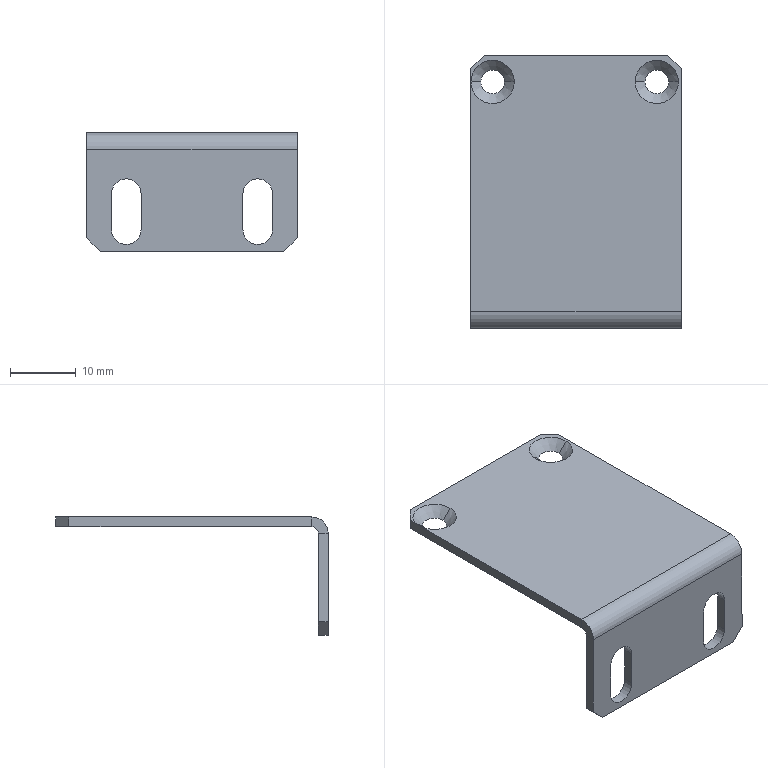Part | STEP file | FBDS-CS-034 | 1 solid | 32 faces | box 32 x 41.5 x 18 mm | volume 2551 mm3 | plane 20 | cylinder 8 | cone 4 | commonest cylinder face diameters 4.5 x6 2 x1 5 x1
STEP:
#1=CARTESIAN_POINT('',(-7.75,-21.5,-9.25));
#2=VERTEX_POINT('',#1);
#3=CARTESIAN_POINT('',(-10.,-21.5,-7.));
#4=VERTEX_POINT('',#3);
#5=CARTESIAN_POINT('',(-10.,-21.5,-9.25));
#6=DIRECTION('',(0.,-1.,0.));
#7=DIRECTION('',(0.,0.,-1.));
#8=AXIS2_PLACEMENT_3D('',#5,#6,#7);
#9=CIRCLE('',#8,2.25);
#10=EDGE_CURVE('',#2,#4,#9,.T.);
#11=ORIENTED_EDGE('',*,*,#10,.T.);
#12=CARTESIAN_POINT('',(-10.,-20.,-7.));
#13=VERTEX_POINT('',#12);
#14=CARTESIAN_POINT('',(-10.,-20.,-7.));
#15=DIRECTION('',(0.,1.,0.));
#16=VECTOR('',#15,1000.);
#17=LINE('',#14,#16);
#18=EDGE_CURVE('',#4,#13,#17,.T.);
#19=ORIENTED_EDGE('',*,*,#18,.T.);
#20=CARTESIAN_POINT('',(-7.75,-20.,-9.25));
#21=VERTEX_POINT('',#20);
#22=CARTESIAN_POINT('',(-10.,-20.,-9.25));
#23=DIRECTION('',(0.,1.,0.));
#24=DIRECTION('',(0.,0.,1.));
#25=AXIS2_PLACEMENT_3D('',#22,#23,#24);
#26=CIRCLE('',#25,2.25);
#27=EDGE_CURVE('',#13,#21,#26,.T.);
#28=ORIENTED_EDGE('',*,*,#27,.T.);
#29=CARTESIAN_POINT('',(-7.75,-30.1,-9.25));
#30=DIRECTION('',(0.,-1.,0.));
#31=VECTOR('',#30,1000.);
#32=LINE('',#29,#31);
#33=EDGE_CURVE('',#21,#2,#32,.T.);
#34=ORIENTED_EDGE('',*,*,#33,.T.);
#35=EDGE_LOOP('',(#11,#19,#28,#34));
#36=FACE_OUTER_BOUND('',#35,.T.);
#37=CARTESIAN_POINT('',(-10.,-20.,-9.25));
#38=DIRECTION('',(0.,1.,0.));
#39=DIRECTION('',(0.,0.,1.));
#40=AXIS2_PLACEMENT_3D('',#37,#38,#39);
#41=CYLINDRICAL_SURFACE('',#40,2.25);
#42=ADVANCED_FACE('',(#36),#41,.F.);
#43=CARTESIAN_POINT('',(12.25,-21.5,-9.25));
#44=VERTEX_POINT('',#43);
#45=CARTESIAN_POINT('',(10.,-21.5,-7.));
#46=VERTEX_POINT('',#45);
#47=CARTESIAN_POINT('',(10.,-21.5,-9.25));
#48=DIRECTION('',(0.,-1.,0.));
#49=DIRECTION('',(0.,0.,-1.));
#50=AXIS2_PLACEMENT_3D('',#47,#48,#49);
#51=CIRCLE('',#50,2.25);
#52=EDGE_CURVE('',#44,#46,#51,.T.);
#53=ORIENTED_EDGE('',*,*,#52,.T.);
#54=CARTESIAN_POINT('',(10.,-20.,-7.));
#55=VERTEX_POINT('',#54);
#56=CARTESIAN_POINT('',(10.,-20.,-7.));
#57=DIRECTION('',(0.,1.,0.));
#58=VECTOR('',#57,1000.);
#59=LINE('',#56,#58);
#60=EDGE_CURVE('',#46,#55,#59,.T.);
#61=ORIENTED_EDGE('',*,*,#60,.T.);
#62=CARTESIAN_POINT('',(12.25,-20.,-9.25));
#63=VERTEX_POINT('',#62);
#64=CARTESIAN_POINT('',(10.,-20.,-9.25));
#65=DIRECTION('',(0.,1.,0.));
#66=DIRECTION('',(0.,0.,1.));
#67=AXIS2_PLACEMENT_3D('',#64,#65,#66);
#68=CIRCLE('',#67,2.25);
#69=EDGE_CURVE('',#55,#63,#68,.T.);
#70=ORIENTED_EDGE('',*,*,#69,.T.);
#71=CARTESIAN_POINT('',(12.25,-30.1,-9.25));
#72=DIRECTION('',(0.,-1.,0.));
#73=VECTOR('',#72,1000.);
#74=LINE('',#71,#73);
#75=EDGE_CURVE('',#63,#44,#74,.T.);
#76=ORIENTED_EDGE('',*,*,#75,.T.);
#77=EDGE_LOOP('',(#53,#61,#70,#76));
#78=FACE_OUTER_BOUND('',#77,.T.);
#79=CARTESIAN_POINT('',(10.,-20.,-9.25));
#80=DIRECTION('',(0.,1.,0.));
#81=DIRECTION('',(0.,0.,1.));
#82=AXIS2_PLACEMENT_3D('',#79,#80,#81);
#83=CYLINDRICAL_SURFACE('',#82,2.25);
#84=ADVANCED_FACE('',(#78),#83,.F.);
#85=CARTESIAN_POINT('',(-10.9,16.,-1.5));
#86=VERTEX_POINT('',#85);
#87=CARTESIAN_POINT('',(-14.5,16.,-1.5));
#88=VERTEX_POINT('',#87);
#89=CARTESIAN_POINT('',(-12.7,16.,-1.5));
#90=DIRECTION('',(0.,0.,-1.));
#91=DIRECTION('',(-1.,0.,0.));
#92=AXIS2_PLACEMENT_3D('',#89,#90,#91);
#93=CIRCLE('',#92,1.8);
#94=EDGE_CURVE('',#86,#88,#93,.T.);
#95=ORIENTED_EDGE('',*,*,#94,.T.);
#96=CARTESIAN_POINT('',(-16.,16.,0.));
#97=VERTEX_POINT('',#96);
#98=CARTESIAN_POINT('',(-16.,16.,0.));
#99=DIRECTION('',(-0.7071,0.,0.7071));
#100=VECTOR('',#99,1000.);
#101=LINE('',#98,#100);
#102=EDGE_CURVE('',#88,#97,#101,.T.);
#103=ORIENTED_EDGE('',*,*,#102,.T.);
#104=CARTESIAN_POINT('',(-9.4,16.,0.));
#105=VERTEX_POINT('',#104);
#106=CARTESIAN_POINT('',(-12.7,16.,0.));
#107=DIRECTION('',(0.,0.,1.));
#108=DIRECTION('',(1.,0.,0.));
#109=AXIS2_PLACEMENT_3D('',#106,#107,#108);
#110=CIRCLE('',#109,3.3);
#111=EDGE_CURVE('',#97,#105,#110,.T.);
#112=ORIENTED_EDGE('',*,*,#111,.T.);
#113=CARTESIAN_POINT('',(-9.4,16.,0.));
#114=DIRECTION('',(0.7071,0.,0.7071));
#115=VECTOR('',#114,1000.);
#116=LINE('',#113,#115);
#117=EDGE_CURVE('',#86,#105,#116,.T.);
#118=ORIENTED_EDGE('',*,*,#117,.F.);
#119=EDGE_LOOP('',(#95,#103,#112,#118));
#120=FACE_OUTER_BOUND('',#119,.T.);
#121=CARTESIAN_POINT('',(-12.7,16.,0.));
#122=DIRECTION('',(0.,0.,1.));
#123=DIRECTION('',(1.,0.,0.));
#124=AXIS2_PLACEMENT_3D('',#121,#122,#123);
#125=CONICAL_SURFACE('',#124,3.3,0.7854);
#126=ADVANCED_FACE('',(#120),#125,.F.);
#127=CARTESIAN_POINT('',(14.1,16.,-1.5));
#128=VERTEX_POINT('',#127);
#129=CARTESIAN_POINT('',(10.5,16.,-1.5));
#130=VERTEX_POINT('',#129);
#131=CARTESIAN_POINT('',(12.3,16.,-1.5));
#132=DIRECTION('',(0.,0.,-1.));
#133=DIRECTION('',(-1.,0.,0.));
#134=AXIS2_PLACEMENT_3D('',#131,#132,#133);
#135=CIRCLE('',#134,1.8);
#136=EDGE_CURVE('',#128,#130,#135,.T.);
#137=ORIENTED_EDGE('',*,*,#136,.T.);
#138=CARTESIAN_POINT('',(9.,16.,0.));
#139=VERTEX_POINT('',#138);
#140=CARTESIAN_POINT('',(9.,16.,0.));
#141=DIRECTION('',(-0.7071,0.,0.7071));
#142=VECTOR('',#141,1000.);
#143=LINE('',#140,#142);
#144=EDGE_CURVE('',#130,#139,#143,.T.);
#145=ORIENTED_EDGE('',*,*,#144,.T.);
#146=CARTESIAN_POINT('',(15.6,16.,0.));
#147=VERTEX_POINT('',#146);
#148=CARTESIAN_POINT('',(12.3,16.,0.));
#149=DIRECTION('',(0.,0.,1.));
#150=DIRECTION('',(1.,0.,0.));
#151=AXIS2_PLACEMENT_3D('',#148,#149,#150);
#152=CIRCLE('',#151,3.3);
#153=EDGE_CURVE('',#139,#147,#152,.T.);
#154=ORIENTED_EDGE('',*,*,#153,.T.);
#155=CARTESIAN_POINT('',(15.6,16.,0.));
#156=DIRECTION('',(0.7071,0.,0.7071));
#157=VECTOR('',#156,1000.);
#158=LINE('',#155,#157);
#159=EDGE_CURVE('',#128,#147,#158,.T.);
#160=ORIENTED_EDGE('',*,*,#159,.F.);
#161=EDGE_LOOP('',(#137,#145,#154,#160));
#162=FACE_OUTER_BOUND('',#161,.T.);
#163=CARTESIAN_POINT('',(12.3,16.,0.));
#164=DIRECTION('',(0.,0.,1.));
#165=DIRECTION('',(1.,0.,0.));
#166=AXIS2_PLACEMENT_3D('',#163,#164,#165);
#167=CONICAL_SURFACE('',#166,3.3,0.7854);
#168=ADVANCED_FACE('',(#162),#167,.F.);
#169=CARTESIAN_POINT('',(16.,-20.,-2.5));
#170=VERTEX_POINT('',#169);
#171=CARTESIAN_POINT('',(16.,-20.,-16.));
#172=VERTEX_POINT('',#171);
#173=CARTESIAN_POINT('',(16.,-20.,-18.));
#174=DIRECTION('',(0.,0.,-1.));
#175=VECTOR('',#174,1000.);
#176=LINE('',#173,#175);
#177=EDGE_CURVE('',#170,#172,#176,.T.);
#178=ORIENTED_EDGE('',*,*,#177,.T.);
#179=CARTESIAN_POINT('',(14.,-20.,-18.));
#180=VERTEX_POINT('',#179);
#181=CARTESIAN_POINT('',(16.,-20.,-16.));
#182=DIRECTION('',(-0.7071,0.,-0.7071));
#183=VECTOR('',#182,1000.);
#184=LINE('',#181,#183);
#185=EDGE_CURVE('',#172,#180,#184,.T.);
#186=ORIENTED_EDGE('',*,*,#185,.T.);
#187=CARTESIAN_POINT('',(-14.,-20.,-18.));
#188=VERTEX_POINT('',#187);
#189=CARTESIAN_POINT('',(-16.,-20.,-18.));
#190=DIRECTION('',(-1.,0.,0.));
#191=VECTOR('',#190,1000.);
#192=LINE('',#189,#191);
#193=EDGE_CURVE('',#180,#188,#192,.T.);
#194=ORIENTED_EDGE('',*,*,#193,.T.);
#195=CARTESIAN_POINT('',(-16.,-20.,-16.));
#196=VERTEX_POINT('',#195);
#197=CARTESIAN_POINT('',(-14.,-20.,-18.));
#198=DIRECTION('',(-0.7071,0.,0.7071));
#199=VECTOR('',#198,1000.);
#200=LINE('',#197,#199);
#201=EDGE_CURVE('',#188,#196,#200,.T.);
#202=ORIENTED_EDGE('',*,*,#201,.T.);
#203=CARTESIAN_POINT('',(-16.,-20.,-2.5));
#204=VERTEX_POINT('',#203);
#205=CARTESIAN_POINT('',(-16.,-20.,-1.5));
#206=DIRECTION('',(0.,0.,1.));
#207=VECTOR('',#206,1000.);
#208=LINE('',#205,#207);
#209=EDGE_CURVE('',#196,#204,#208,.T.);
#210=ORIENTED_EDGE('',*,*,#209,.T.);
#211=CARTESIAN_POINT('',(16.,-20.,-2.5));
#212=DIRECTION('',(-1.,0.,0.));
#213=VECTOR('',#212,1000.);
#214=LINE('',#211,#213);
#215=EDGE_CURVE('',#170,#204,#214,.T.);
#216=ORIENTED_EDGE('',*,*,#215,.F.);
#217=EDGE_LOOP('',(#178,#186,#194,#202,#210,#216));
#218=FACE_OUTER_BOUND('',#217,.T.);
#219=CARTESIAN_POINT('',(12.25,-20.,-14.75));
#220=VERTEX_POINT('',#219);
#221=CARTESIAN_POINT('',(7.75,-20.,-14.75));
#222=VERTEX_POINT('',#221);
#223=CARTESIAN_POINT('',(10.,-20.,-14.75));
#224=DIRECTION('',(0.,1.,0.));
#225=DIRECTION('',(0.,0.,1.));
#226=AXIS2_PLACEMENT_3D('',#223,#224,#225);
#227=CIRCLE('',#226,2.25);
#228=EDGE_CURVE('',#220,#222,#227,.T.);
#229=ORIENTED_EDGE('',*,*,#228,.F.);
#230=CARTESIAN_POINT('',(12.25,-20.,-9.25));
#231=DIRECTION('',(0.,0.,-1.));
#232=VECTOR('',#231,1000.);
#233=LINE('',#230,#232);
#234=EDGE_CURVE('',#63,#220,#233,.T.);
#235=ORIENTED_EDGE('',*,*,#234,.F.);
#236=ORIENTED_EDGE('',*,*,#69,.F.);
#237=CARTESIAN_POINT('',(7.75,-20.,-9.25));
#238=VERTEX_POINT('',#237);
#239=CARTESIAN_POINT('',(10.,-20.,-9.25));
#240=DIRECTION('',(0.,1.,0.));
#241=DIRECTION('',(0.,0.,1.));
#242=AXIS2_PLACEMENT_3D('',#239,#240,#241);
#243=CIRCLE('',#242,2.25);
#244=EDGE_CURVE('',#238,#55,#243,.T.);
#245=ORIENTED_EDGE('',*,*,#244,.F.);
#246=CARTESIAN_POINT('',(7.75,-20.,-9.25));
#247=DIRECTION('',(0.,0.,-1.));
#248=VECTOR('',#247,1000.);
#249=LINE('',#246,#248);
#250=EDGE_CURVE('',#238,#222,#249,.T.);
#251=ORIENTED_EDGE('',*,*,#250,.T.);
#252=EDGE_LOOP('',(#229,#235,#236,#245,#251));
#253=FACE_BOUND('',#252,.T.);
#254=CARTESIAN_POINT('',(-7.75,-20.,-14.75));
#255=VERTEX_POINT('',#254);
#256=CARTESIAN_POINT('',(-12.25,-20.,-14.75));
#257=VERTEX_POINT('',#256);
#258=CARTESIAN_POINT('',(-10.,-20.,-14.75));
#259=DIRECTION('',(0.,1.,0.));
#260=DIRECTION('',(0.,0.,1.));
#261=AXIS2_PLACEMENT_3D('',#258,#259,#260);
#262=CIRCLE('',#261,2.25);
#263=EDGE_CURVE('',#255,#257,#262,.T.);
#264=ORIENTED_EDGE('',*,*,#263,.F.);
#265=CARTESIAN_POINT('',(-7.75,-20.,-9.25));
#266=DIRECTION('',(0.,0.,-1.));
#267=VECTOR('',#266,1000.);
#268=LINE('',#265,#267);
#269=EDGE_CURVE('',#21,#255,#268,.T.);
#270=ORIENTED_EDGE('',*,*,#269,.F.);
#271=ORIENTED_EDGE('',*,*,#27,.F.);
#272=CARTESIAN_POINT('',(-12.25,-20.,-9.25));
#273=VERTEX_POINT('',#272);
#274=CARTESIAN_POINT('',(-10.,-20.,-9.25));
#275=DIRECTION('',(0.,1.,0.));
#276=DIRECTION('',(0.,0.,1.));
#277=AXIS2_PLACEMENT_3D('',#274,#275,#276);
#278=CIRCLE('',#277,2.25);
#279=EDGE_CURVE('',#273,#13,#278,.T.);
#280=ORIENTED_EDGE('',*,*,#279,.F.);
#281=CARTESIAN_POINT('',(-12.25,-20.,-9.25));
#282=DIRECTION('',(0.,0.,-1.));
#283=VECTOR('',#282,1000.);
#284=LINE('',#281,#283);
#285=EDGE_CURVE('',#273,#257,#284,.T.);
#286=ORIENTED_EDGE('',*,*,#285,.T.);
#287=EDGE_LOOP('',(#264,#270,#271,#280,#286));
#288=FACE_BOUND('',#287,.T.);
#289=CARTESIAN_POINT('',(0.,-20.,0.));
#290=DIRECTION('',(0.,-1.,0.));
#291=DIRECTION('',(0.,0.,-1.));
#292=AXIS2_PLACEMENT_3D('',#289,#290,#291);
#293=PLANE('',#292);
#294=ADVANCED_FACE('',(#218,#253,#288),#293,.F.);
#295=ORIENTED_EDGE('',*,*,#94,.F.);
#296=CARTESIAN_POINT('',(-12.7,16.,-1.5));
#297=DIRECTION('',(0.,0.,-1.));
#298=DIRECTION('',(-1.,0.,0.));
#299=AXIS2_PLACEMENT_3D('',#296,#297,#298);
#300=CIRCLE('',#299,1.8);
#301=EDGE_CURVE('',#88,#86,#300,.T.);
#302=ORIENTED_EDGE('',*,*,#301,.F.);
#303=EDGE_LOOP('',(#295,#302));
#304=FACE_BOUND('',#303,.T.);
#305=ORIENTED_EDGE('',*,*,#136,.F.);
#306=CARTESIAN_POINT('',(12.3,16.,-1.5));
#307=DIRECTION('',(0.,0.,-1.));
#308=DIRECTION('',(-1.,0.,0.));
#309=AXIS2_PLACEMENT_3D('',#306,#307,#308);
#310=CIRCLE('',#309,1.8);
#311=EDGE_CURVE('',#130,#128,#310,.T.);
#312=ORIENTED_EDGE('',*,*,#311,.F.);
#313=EDGE_LOOP('',(#305,#312));
#314=FACE_BOUND('',#313,.T.);
#315=CARTESIAN_POINT('',(-16.,18.,-1.5));
#316=VERTEX_POINT('',#315);
#317=CARTESIAN_POINT('',(-16.,-19.,-1.5));
#318=VERTEX_POINT('',#317);
#319=CARTESIAN_POINT('',(-16.,-20.,-1.5));
#320=DIRECTION('',(0.,-1.,0.));
#321=VECTOR('',#320,1000.);
#322=LINE('',#319,#321);
#323=EDGE_CURVE('',#316,#318,#322,.T.);
#324=ORIENTED_EDGE('',*,*,#323,.F.);
#325=CARTESIAN_POINT('',(-14.,20.,-1.5));
#326=VERTEX_POINT('',#325);
#327=CARTESIAN_POINT('',(-17.,17.,-1.5));
#328=DIRECTION('',(0.7071,0.7071,0.));
#329=VECTOR('',#328,1000.);
#330=LINE('',#327,#329);
#331=EDGE_CURVE('',#316,#326,#330,.T.);
#332=ORIENTED_EDGE('',*,*,#331,.T.);
#333=CARTESIAN_POINT('',(14.,20.,-1.5));
#334=VERTEX_POINT('',#333);
#335=CARTESIAN_POINT('',(-16.,20.,-1.5));
#336=DIRECTION('',(-1.,0.,0.));
#337=VECTOR('',#336,1000.);
#338=LINE('',#335,#337);
#339=EDGE_CURVE('',#334,#326,#338,.T.);
#340=ORIENTED_EDGE('',*,*,#339,.F.);
#341=CARTESIAN_POINT('',(16.,18.,-1.5));
#342=VERTEX_POINT('',#341);
#343=CARTESIAN_POINT('',(17.,17.,-1.5));
#344=DIRECTION('',(0.7071,-0.7071,0.));
#345=VECTOR('',#344,1000.);
#346=LINE('',#343,#345);
#347=EDGE_CURVE('',#334,#342,#346,.T.);
#348=ORIENTED_EDGE('',*,*,#347,.T.);
#349=CARTESIAN_POINT('',(16.,-19.,-1.5));
#350=VERTEX_POINT('',#349);
#351=CARTESIAN_POINT('',(16.,-20.,-1.5));
#352=DIRECTION('',(0.,1.,0.));
#353=VECTOR('',#352,1000.);
#354=LINE('',#351,#353);
#355=EDGE_CURVE('',#350,#342,#354,.T.);
#356=ORIENTED_EDGE('',*,*,#355,.F.);
#357=CARTESIAN_POINT('',(-16.,-19.,-1.5));
#358=DIRECTION('',(1.,0.,0.));
#359=VECTOR('',#358,1000.);
#360=LINE('',#357,#359);
#361=EDGE_CURVE('',#318,#350,#360,.T.);
#362=ORIENTED_EDGE('',*,*,#361,.F.);
#363=EDGE_LOOP('',(#324,#332,#340,#348,#356,#362));
#364=FACE_OUTER_BOUND('',#363,.T.);
#365=CARTESIAN_POINT('',(0.,0.,-1.5));
#366=DIRECTION('',(0.,0.,-1.));
#367=DIRECTION('',(-1.,0.,0.));
#368=AXIS2_PLACEMENT_3D('',#365,#366,#367);
#369=PLANE('',#368);
#370=ADVANCED_FACE('',(#304,#314,#364),#369,.T.);
#371=CARTESIAN_POINT('',(-16.,18.,0.));
#372=VERTEX_POINT('',#371);
#373=CARTESIAN_POINT('',(-16.,-20.,0.));
#374=DIRECTION('',(0.,-1.,0.));
#375=VECTOR('',#374,1000.);
#376=LINE('',#373,#375);
#377=EDGE_CURVE('',#372,#97,#376,.T.);
#378=ORIENTED_EDGE('',*,*,#377,.F.);
#379=CARTESIAN_POINT('',(-16.,18.,-1.5));
#380=DIRECTION('',(0.,0.,-1.));
#381=VECTOR('',#380,1000.);
#382=LINE('',#379,#381);
#383=EDGE_CURVE('',#372,#316,#382,.T.);
#384=ORIENTED_EDGE('',*,*,#383,.T.);
#385=ORIENTED_EDGE('',*,*,#323,.T.);
#386=CARTESIAN_POINT('',(-16.,-19.,0.));
#387=VERTEX_POINT('',#386);
#388=CARTESIAN_POINT('',(-16.,-19.,-1.5));
#389=DIRECTION('',(0.,0.,1.));
#390=VECTOR('',#389,1000.);
#391=LINE('',#388,#390);
#392=EDGE_CURVE('',#318,#387,#391,.T.);
#393=ORIENTED_EDGE('',*,*,#392,.T.);
#394=CARTESIAN_POINT('',(-16.,-20.,0.));
#395=DIRECTION('',(0.,-1.,0.));
#396=VECTOR('',#395,1000.);
#397=LINE('',#394,#396);
#398=EDGE_CURVE('',#97,#387,#397,.T.);
#399=ORIENTED_EDGE('',*,*,#398,.F.);
#400=EDGE_LOOP('',(#378,#384,#385,#393,#399));
#401=FACE_OUTER_BOUND('',#400,.T.);
#402=CARTESIAN_POINT('',(-16.,-20.,-1.5));
#403=DIRECTION('',(-1.,0.,0.));
#404=DIRECTION('',(0.,0.,1.));
#405=AXIS2_PLACEMENT_3D('',#402,#403,#404);
#406=PLANE('',#405);
#407=ADVANCED_FACE('',(#401),#406,.T.);
#408=CARTESIAN_POINT('',(12.3,16.,0.));
#409=DIRECTION('',(0.,0.,1.));
#410=DIRECTION('',(1.,0.,0.));
#411=AXIS2_PLACEMENT_3D('',#408,#409,#410);
#412=CIRCLE('',#411,3.3);
#413=EDGE_CURVE('',#147,#139,#412,.T.);
#414=ORIENTED_EDGE('',*,*,#413,.F.);
#415=ORIENTED_EDGE('',*,*,#153,.F.);
#416=EDGE_LOOP('',(#414,#415));
#417=FACE_BOUND('',#416,.T.);
#418=CARTESIAN_POINT('',(14.,20.,0.));
#419=VERTEX_POINT('',#418);
#420=CARTESIAN_POINT('',(-14.,20.,0.));
#421=VERTEX_POINT('',#420);
#422=CARTESIAN_POINT('',(-16.,20.,0.));
#423=DIRECTION('',(-1.,0.,0.));
#424=VECTOR('',#423,1000.);
#425=LINE('',#422,#424);
#426=EDGE_CURVE('',#419,#421,#425,.T.);
#427=ORIENTED_EDGE('',*,*,#426,.T.);
#428=CARTESIAN_POINT('',(-14.,20.,0.));
#429=DIRECTION('',(-0.7071,-0.7071,0.));
#430=VECTOR('',#429,1000.);
#431=LINE('',#428,#430);
#432=EDGE_CURVE('',#421,#372,#431,.T.);
#433=ORIENTED_EDGE('',*,*,#432,.T.);
#434=ORIENTED_EDGE('',*,*,#377,.T.);
#435=CARTESIAN_POINT('',(-12.7,16.,0.));
#436=DIRECTION('',(0.,0.,1.));
#437=DIRECTION('',(1.,0.,0.));
#438=AXIS2_PLACEMENT_3D('',#435,#436,#437);
#439=CIRCLE('',#438,3.3);
#440=EDGE_CURVE('',#105,#97,#439,.T.);
#441=ORIENTED_EDGE('',*,*,#440,.F.);
#442=ORIENTED_EDGE('',*,*,#111,.F.);
#443=ORIENTED_EDGE('',*,*,#398,.T.);
#444=CARTESIAN_POINT('',(16.,-19.,0.));
#445=VERTEX_POINT('',#444);
#446=CARTESIAN_POINT('',(-16.,-19.,0.));
#447=DIRECTION('',(1.,0.,0.));
#448=VECTOR('',#447,1000.);
#449=LINE('',#446,#448);
#450=EDGE_CURVE('',#387,#445,#449,.T.);
#451=ORIENTED_EDGE('',*,*,#450,.T.);
#452=CARTESIAN_POINT('',(16.,18.,0.));
#453=VERTEX_POINT('',#452);
#454=CARTESIAN_POINT('',(16.,-20.,0.));
#455=DIRECTION('',(0.,1.,0.));
#456=VECTOR('',#455,1000.);
#457=LINE('',#454,#456);
#458=EDGE_CURVE('',#445,#453,#457,.T.);
#459=ORIENTED_EDGE('',*,*,#458,.T.);
#460=CARTESIAN_POINT('',(16.,18.,0.));
#461=DIRECTION('',(-0.7071,0.7071,0.));
#462=VECTOR('',#461,1000.);
#463=LINE('',#460,#462);
#464=EDGE_CURVE('',#453,#419,#463,.T.);
#465=ORIENTED_EDGE('',*,*,#464,.T.);
#466=EDGE_LOOP('',(#427,#433,#434,#441,#442,#443,#451,#459,#465));
#467=FACE_OUTER_BOUND('',#466,.T.);
#468=CARTESIAN_POINT('',(0.,0.,0.));
#469=DIRECTION('',(0.,0.,-1.));
#470=DIRECTION('',(-1.,0.,0.));
#471=AXIS2_PLACEMENT_3D('',#468,#469,#470);
#472=PLANE('',#471);
#473=ADVANCED_FACE('',(#417,#467),#472,.F.);
#474=ORIENTED_EDGE('',*,*,#355,.T.);
#475=CARTESIAN_POINT('',(16.,18.,-1.5));
#476=DIRECTION('',(0.,0.,1.));
#477=VECTOR('',#476,1000.);
#478=LINE('',#475,#477);
#479=EDGE_CURVE('',#342,#453,#478,.T.);
#480=ORIENTED_EDGE('',*,*,#479,.T.);
#481=ORIENTED_EDGE('',*,*,#458,.F.);
#482=CARTESIAN_POINT('',(16.,-19.,-1.5));
#483=DIRECTION('',(0.,0.,1.));
#484=VECTOR('',#483,1000.);
#485=LINE('',#482,#484);
#486=EDGE_CURVE('',#350,#445,#485,.T.);
#487=ORIENTED_EDGE('',*,*,#486,.F.);
#488=EDGE_LOOP('',(#474,#480,#481,#487));
#489=FACE_OUTER_BOUND('',#488,.T.);
#490=CARTESIAN_POINT('',(16.,-20.,-1.5));
#491=DIRECTION('',(1.,0.,0.));
#492=DIRECTION('',(0.,0.,-1.));
#493=AXIS2_PLACEMENT_3D('',#490,#491,#492);
#494=PLANE('',#493);
#495=ADVANCED_FACE('',(#489),#494,.T.);
#496=ORIENTED_EDGE('',*,*,#339,.T.);
#497=CARTESIAN_POINT('',(-14.,20.,-1.5));
#498=DIRECTION('',(0.,0.,1.));
#499=VECTOR('',#498,1000.);
#500=LINE('',#497,#499);
#501=EDGE_CURVE('',#326,#421,#500,.T.);
#502=ORIENTED_EDGE('',*,*,#501,.T.);
#503=ORIENTED_EDGE('',*,*,#426,.F.);
#504=CARTESIAN_POINT('',(14.,20.,-1.5));
#505=DIRECTION('',(0.,0.,-1.));
#506=VECTOR('',#505,1000.);
#507=LINE('',#504,#506);
#508=EDGE_CURVE('',#419,#334,#507,.T.);
#509=ORIENTED_EDGE('',*,*,#508,.T.);
#510=EDGE_LOOP('',(#496,#502,#503,#509));
#511=FACE_OUTER_BOUND('',#510,.T.);
#512=CARTESIAN_POINT('',(-16.,20.,-1.5));
#513=DIRECTION('',(0.,1.,0.));
#514=DIRECTION('',(0.,0.,1.));
#515=AXIS2_PLACEMENT_3D('',#512,#513,#514);
#516=PLANE('',#515);
#517=ADVANCED_FACE('',(#511),#516,.T.);
#518=ORIENTED_EDGE('',*,*,#144,.F.);
#519=ORIENTED_EDGE('',*,*,#311,.T.);
#520=ORIENTED_EDGE('',*,*,#159,.T.);
#521=ORIENTED_EDGE('',*,*,#413,.T.);
#522=EDGE_LOOP('',(#518,#519,#520,#521));
#523=FACE_OUTER_BOUND('',#522,.T.);
#524=CARTESIAN_POINT('',(12.3,16.,0.));
#525=DIRECTION('',(0.,0.,1.));
#526=DIRECTION('',(1.,0.,0.));
#527=AXIS2_PLACEMENT_3D('',#524,#525,#526);
#528=CONICAL_SURFACE('',#527,3.3,0.7854);
#529=ADVANCED_FACE('',(#523),#528,.F.);
#530=ORIENTED_EDGE('',*,*,#102,.F.);
#531=ORIENTED_EDGE('',*,*,#301,.T.);
#532=ORIENTED_EDGE('',*,*,#117,.T.);
#533=ORIENTED_EDGE('',*,*,#440,.T.);
#534=EDGE_LOOP('',(#530,#531,#532,#533));
#535=FACE_OUTER_BOUND('',#534,.T.);
#536=CARTESIAN_POINT('',(-12.7,16.,0.));
#537=DIRECTION('',(0.,0.,1.));
#538=DIRECTION('',(1.,0.,0.));
#539=AXIS2_PLACEMENT_3D('',#536,#537,#538);
#540=CONICAL_SURFACE('',#539,3.3,0.7854);
#541=ADVANCED_FACE('',(#535),#540,.F.);
#542=CARTESIAN_POINT('',(16.,-21.5,-2.5));
#543=VERTEX_POINT('',#542);
#544=CARTESIAN_POINT('',(16.,-20.,-2.5));
#545=DIRECTION('',(0.,-1.,0.));
#546=VECTOR('',#545,1000.);
#547=LINE('',#544,#546);
#548=EDGE_CURVE('',#170,#543,#547,.T.);
#549=ORIENTED_EDGE('',*,*,#548,.F.);
#550=CARTESIAN_POINT('',(16.,-19.,-2.5));
#551=DIRECTION('',(1.,0.,0.));
#552=DIRECTION('',(0.,0.,1.));
#553=AXIS2_PLACEMENT_3D('',#550,#551,#552);
#554=CIRCLE('',#553,1.);
#555=EDGE_CURVE('',#350,#170,#554,.T.);
#556=ORIENTED_EDGE('',*,*,#555,.F.);
#557=ORIENTED_EDGE('',*,*,#486,.T.);
#558=CARTESIAN_POINT('',(16.,-19.,-2.5));
#559=DIRECTION('',(1.,0.,0.));
#560=DIRECTION('',(0.,0.,1.));
#561=AXIS2_PLACEMENT_3D('',#558,#559,#560);
#562=CIRCLE('',#561,2.5);
#563=EDGE_CURVE('',#445,#543,#562,.T.);
#564=ORIENTED_EDGE('',*,*,#563,.T.);
#565=EDGE_LOOP('',(#549,#556,#557,#564));
#566=FACE_OUTER_BOUND('',#565,.T.);
#567=CARTESIAN_POINT('',(16.,-19.,-2.5));
#568=DIRECTION('',(1.,0.,0.));
#569=DIRECTION('',(0.,0.,-1.));
#570=AXIS2_PLACEMENT_3D('',#567,#568,#569);
#571=PLANE('',#570);
#572=ADVANCED_FACE('',(#566),#571,.T.);
#573=CARTESIAN_POINT('',(-16.,-19.,-2.5));
#574=DIRECTION('',(-1.,0.,0.));
#575=DIRECTION('',(0.,0.,1.));
#576=AXIS2_PLACEMENT_3D('',#573,#574,#575);
#577=CIRCLE('',#576,1.);
#578=EDGE_CURVE('',#204,#318,#577,.T.);
#579=ORIENTED_EDGE('',*,*,#578,.F.);
#580=CARTESIAN_POINT('',(-16.,-21.5,-2.5));
#581=VERTEX_POINT('',#580);
#582=CARTESIAN_POINT('',(-16.,-20.,-2.5));
#583=DIRECTION('',(0.,-1.,0.));
#584=VECTOR('',#583,1000.);
#585=LINE('',#582,#584);
#586=EDGE_CURVE('',#204,#581,#585,.T.);
#587=ORIENTED_EDGE('',*,*,#586,.T.);
#588=CARTESIAN_POINT('',(-16.,-19.,-2.5));
#589=DIRECTION('',(-1.,0.,0.));
#590=DIRECTION('',(0.,0.,1.));
#591=AXIS2_PLACEMENT_3D('',#588,#589,#590);
#592=CIRCLE('',#591,2.5);
#593=EDGE_CURVE('',#581,#387,#592,.T.);
#594=ORIENTED_EDGE('',*,*,#593,.T.);
#595=ORIENTED_EDGE('',*,*,#392,.F.);
#596=EDGE_LOOP('',(#579,#587,#594,#595));
#597=FACE_OUTER_BOUND('',#596,.T.);
#598=CARTESIAN_POINT('',(-16.,-19.,-2.5));
#599=DIRECTION('',(1.,0.,0.));
#600=DIRECTION('',(0.,0.,-1.));
#601=AXIS2_PLACEMENT_3D('',#598,#599,#600);
#602=PLANE('',#601);
#603=ADVANCED_FACE('',(#597),#602,.F.);
#604=ORIENTED_EDGE('',*,*,#450,.F.);
#605=ORIENTED_EDGE('',*,*,#593,.F.);
#606=CARTESIAN_POINT('',(0.,-21.5,-2.5));
#607=DIRECTION('',(-1.,0.,0.));
#608=VECTOR('',#607,1000.);
#609=LINE('',#606,#608);
#610=EDGE_CURVE('',#543,#581,#609,.T.);
#611=ORIENTED_EDGE('',*,*,#610,.F.);
#612=ORIENTED_EDGE('',*,*,#563,.F.);
#613=EDGE_LOOP('',(#604,#605,#611,#612));
#614=FACE_OUTER_BOUND('',#613,.T.);
#615=CARTESIAN_POINT('',(-16.,-19.,-2.5));
#616=DIRECTION('',(-1.,0.,0.));
#617=DIRECTION('',(0.,-1.,0.));
#618=AXIS2_PLACEMENT_3D('',#615,#616,#617);
#619=CYLINDRICAL_SURFACE('',#618,2.5);
#620=ADVANCED_FACE('',(#614),#619,.T.);
#621=ORIENTED_EDGE('',*,*,#361,.T.);
#622=ORIENTED_EDGE('',*,*,#555,.T.);
#623=ORIENTED_EDGE('',*,*,#215,.T.);
#624=ORIENTED_EDGE('',*,*,#578,.T.);
#625=EDGE_LOOP('',(#621,#622,#623,#624));
#626=FACE_OUTER_BOUND('',#625,.T.);
#627=CARTESIAN_POINT('',(-16.,-19.,-2.5));
#628=DIRECTION('',(-1.,0.,0.));
#629=DIRECTION('',(0.,-1.,0.));
#630=AXIS2_PLACEMENT_3D('',#627,#628,#629);
#631=CYLINDRICAL_SURFACE('',#630,1.);
#632=ADVANCED_FACE('',(#626),#631,.F.);
#633=ORIENTED_EDGE('',*,*,#209,.F.);
#634=CARTESIAN_POINT('',(-16.,-21.5,-16.));
#635=VERTEX_POINT('',#634);
#636=CARTESIAN_POINT('',(-16.,-21.5,-16.));
#637=DIRECTION('',(0.,-1.,0.));
#638=VECTOR('',#637,1000.);
#639=LINE('',#636,#638);
#640=EDGE_CURVE('',#196,#635,#639,.T.);
#641=ORIENTED_EDGE('',*,*,#640,.T.);
#642=CARTESIAN_POINT('',(-16.,-21.5,-1.5));
#643=DIRECTION('',(0.,0.,1.));
#644=VECTOR('',#643,1000.);
#645=LINE('',#642,#644);
#646=EDGE_CURVE('',#635,#581,#645,.T.);
#647=ORIENTED_EDGE('',*,*,#646,.T.);
#648=ORIENTED_EDGE('',*,*,#586,.F.);
#649=EDGE_LOOP('',(#633,#641,#647,#648));
#650=FACE_OUTER_BOUND('',#649,.T.);
#651=CARTESIAN_POINT('',(-16.,-21.5,-1.5));
#652=DIRECTION('',(-1.,0.,0.));
#653=DIRECTION('',(0.,0.,1.));
#654=AXIS2_PLACEMENT_3D('',#651,#652,#653);
#655=PLANE('',#654);
#656=ADVANCED_FACE('',(#650),#655,.T.);
#657=CARTESIAN_POINT('',(16.,-21.5,-16.));
#658=VERTEX_POINT('',#657);
#659=CARTESIAN_POINT('',(16.,-21.5,-18.));
#660=DIRECTION('',(0.,0.,-1.));
#661=VECTOR('',#660,1000.);
#662=LINE('',#659,#661);
#663=EDGE_CURVE('',#543,#658,#662,.T.);
#664=ORIENTED_EDGE('',*,*,#663,.T.);
#665=CARTESIAN_POINT('',(16.,-21.5,-16.));
#666=DIRECTION('',(0.,1.,0.));
#667=VECTOR('',#666,1000.);
#668=LINE('',#665,#667);
#669=EDGE_CURVE('',#658,#172,#668,.T.);
#670=ORIENTED_EDGE('',*,*,#669,.T.);
#671=ORIENTED_EDGE('',*,*,#177,.F.);
#672=ORIENTED_EDGE('',*,*,#548,.T.);
#673=EDGE_LOOP('',(#664,#670,#671,#672));
#674=FACE_OUTER_BOUND('',#673,.T.);
#675=CARTESIAN_POINT('',(16.,-21.5,-18.));
#676=DIRECTION('',(1.,0.,0.));
#677=DIRECTION('',(0.,0.,-1.));
#678=AXIS2_PLACEMENT_3D('',#675,#676,#677);
#679=PLANE('',#678);
#680=ADVANCED_FACE('',(#674),#679,.T.);
#681=CARTESIAN_POINT('',(-12.25,-21.5,-14.75));
#682=VERTEX_POINT('',#681);
#683=CARTESIAN_POINT('',(-7.75,-21.5,-14.75));
#684=VERTEX_POINT('',#683);
#685=CARTESIAN_POINT('',(-10.,-21.5,-14.75));
#686=DIRECTION('',(0.,-1.,0.));
#687=DIRECTION('',(0.,0.,-1.));
#688=AXIS2_PLACEMENT_3D('',#685,#686,#687);
#689=CIRCLE('',#688,2.25);
#690=EDGE_CURVE('',#682,#684,#689,.T.);
#691=ORIENTED_EDGE('',*,*,#690,.F.);
#692=CARTESIAN_POINT('',(-12.25,-21.5,-9.25));
#693=VERTEX_POINT('',#692);
#694=CARTESIAN_POINT('',(-12.25,-21.5,0.));
#695=DIRECTION('',(0.,0.,-1.));
#696=VECTOR('',#695,1000.);
#697=LINE('',#694,#696);
#698=EDGE_CURVE('',#693,#682,#697,.T.);
#699=ORIENTED_EDGE('',*,*,#698,.F.);
#700=CARTESIAN_POINT('',(-10.,-21.5,-9.25));
#701=DIRECTION('',(0.,-1.,0.));
#702=DIRECTION('',(0.,0.,-1.));
#703=AXIS2_PLACEMENT_3D('',#700,#701,#702);
#704=CIRCLE('',#703,2.25);
#705=EDGE_CURVE('',#4,#693,#704,.T.);
#706=ORIENTED_EDGE('',*,*,#705,.F.);
#707=ORIENTED_EDGE('',*,*,#10,.F.);
#708=CARTESIAN_POINT('',(-7.75,-21.5,0.));
#709=DIRECTION('',(0.,0.,1.));
#710=VECTOR('',#709,1000.);
#711=LINE('',#708,#710);
#712=EDGE_CURVE('',#684,#2,#711,.T.);
#713=ORIENTED_EDGE('',*,*,#712,.F.);
#714=EDGE_LOOP('',(#691,#699,#706,#707,#713));
#715=FACE_BOUND('',#714,.T.);
#716=CARTESIAN_POINT('',(7.75,-21.5,-9.25));
#717=VERTEX_POINT('',#716);
#718=CARTESIAN_POINT('',(7.75,-21.5,-14.75));
#719=VERTEX_POINT('',#718);
#720=CARTESIAN_POINT('',(7.75,-21.5,0.));
#721=DIRECTION('',(0.,0.,-1.));
#722=VECTOR('',#721,1000.);
#723=LINE('',#720,#722);
#724=EDGE_CURVE('',#717,#719,#723,.T.);
#725=ORIENTED_EDGE('',*,*,#724,.F.);
#726=CARTESIAN_POINT('',(10.,-21.5,-9.25));
#727=DIRECTION('',(0.,-1.,0.));
#728=DIRECTION('',(0.,0.,-1.));
#729=AXIS2_PLACEMENT_3D('',#726,#727,#728);
#730=CIRCLE('',#729,2.25);
#731=EDGE_CURVE('',#46,#717,#730,.T.);
#732=ORIENTED_EDGE('',*,*,#731,.F.);
#733=ORIENTED_EDGE('',*,*,#52,.F.);
#734=CARTESIAN_POINT('',(12.25,-21.5,-14.75));
#735=VERTEX_POINT('',#734);
#736=CARTESIAN_POINT('',(12.25,-21.5,0.));
#737=DIRECTION('',(0.,0.,1.));
#738=VECTOR('',#737,1000.);
#739=LINE('',#736,#738);
#740=EDGE_CURVE('',#735,#44,#739,.T.);
#741=ORIENTED_EDGE('',*,*,#740,.F.);
#742=CARTESIAN_POINT('',(10.,-21.5,-14.75));
#743=DIRECTION('',(0.,-1.,0.));
#744=DIRECTION('',(0.,0.,-1.));
#745=AXIS2_PLACEMENT_3D('',#742,#743,#744);
#746=CIRCLE('',#745,2.25);
#747=EDGE_CURVE('',#719,#735,#746,.T.);
#748=ORIENTED_EDGE('',*,*,#747,.F.);
#749=EDGE_LOOP('',(#725,#732,#733,#741,#748));
#750=FACE_BOUND('',#749,.T.);
#751=CARTESIAN_POINT('',(14.,-21.5,-18.));
#752=VERTEX_POINT('',#751);
#753=CARTESIAN_POINT('',(-14.,-21.5,-18.));
#754=VERTEX_POINT('',#753);
#755=CARTESIAN_POINT('',(-16.,-21.5,-18.));
#756=DIRECTION('',(-1.,0.,0.));
#757=VECTOR('',#756,1000.);
#758=LINE('',#755,#757);
#759=EDGE_CURVE('',#752,#754,#758,.T.);
#760=ORIENTED_EDGE('',*,*,#759,.F.);
#761=CARTESIAN_POINT('',(16.,-21.5,-16.));
#762=DIRECTION('',(0.7071,0.,0.7071));
#763=VECTOR('',#762,1000.);
#764=LINE('',#761,#763);
#765=EDGE_CURVE('',#752,#658,#764,.T.);
#766=ORIENTED_EDGE('',*,*,#765,.T.);
#767=ORIENTED_EDGE('',*,*,#663,.F.);
#768=ORIENTED_EDGE('',*,*,#610,.T.);
#769=ORIENTED_EDGE('',*,*,#646,.F.);
#770=CARTESIAN_POINT('',(-16.,-21.5,-16.));
#771=DIRECTION('',(0.7071,0.,-0.7071));
#772=VECTOR('',#771,1000.);
#773=LINE('',#770,#772);
#774=EDGE_CURVE('',#635,#754,#773,.T.);
#775=ORIENTED_EDGE('',*,*,#774,.T.);
#776=EDGE_LOOP('',(#760,#766,#767,#768,#769,#775));
#777=FACE_OUTER_BOUND('',#776,.T.);
#778=CARTESIAN_POINT('',(0.,-21.5,0.));
#779=DIRECTION('',(0.,-1.,0.));
#780=DIRECTION('',(0.,0.,-1.));
#781=AXIS2_PLACEMENT_3D('',#778,#779,#780);
#782=PLANE('',#781);
#783=ADVANCED_FACE('',(#715,#750,#777),#782,.T.);
#784=ORIENTED_EDGE('',*,*,#193,.F.);
#785=CARTESIAN_POINT('',(14.,-21.5,-18.));
#786=DIRECTION('',(0.,-1.,0.));
#787=VECTOR('',#786,1000.);
#788=LINE('',#785,#787);
#789=EDGE_CURVE('',#180,#752,#788,.T.);
#790=ORIENTED_EDGE('',*,*,#789,.T.);
#791=ORIENTED_EDGE('',*,*,#759,.T.);
#792=CARTESIAN_POINT('',(-14.,-21.5,-18.));
#793=DIRECTION('',(0.,1.,0.));
#794=VECTOR('',#793,1000.);
#795=LINE('',#792,#794);
#796=EDGE_CURVE('',#754,#188,#795,.T.);
#797=ORIENTED_EDGE('',*,*,#796,.T.);
#798=EDGE_LOOP('',(#784,#790,#791,#797));
#799=FACE_OUTER_BOUND('',#798,.T.);
#800=CARTESIAN_POINT('',(-16.,-21.5,-18.));
#801=DIRECTION('',(0.,0.,-1.));
#802=DIRECTION('',(0.,1.,0.));
#803=AXIS2_PLACEMENT_3D('',#800,#801,#802);
#804=PLANE('',#803);
#805=ADVANCED_FACE('',(#799),#804,.T.);
#806=ORIENTED_EDGE('',*,*,#747,.T.);
#807=CARTESIAN_POINT('',(12.25,-30.1,-14.75));
#808=DIRECTION('',(0.,-1.,0.));
#809=VECTOR('',#808,1000.);
#810=LINE('',#807,#809);
#811=EDGE_CURVE('',#220,#735,#810,.T.);
#812=ORIENTED_EDGE('',*,*,#811,.F.);
#813=ORIENTED_EDGE('',*,*,#228,.T.);
#814=CARTESIAN_POINT('',(7.75,-20.,-14.75));
#815=DIRECTION('',(0.,1.,0.));
#816=VECTOR('',#815,1000.);
#817=LINE('',#814,#816);
#818=EDGE_CURVE('',#719,#222,#817,.T.);
#819=ORIENTED_EDGE('',*,*,#818,.F.);
#820=EDGE_LOOP('',(#806,#812,#813,#819));
#821=FACE_OUTER_BOUND('',#820,.T.);
#822=CARTESIAN_POINT('',(10.,-20.,-14.75));
#823=DIRECTION('',(0.,1.,0.));
#824=DIRECTION('',(0.,0.,1.));
#825=AXIS2_PLACEMENT_3D('',#822,#823,#824);
#826=CYLINDRICAL_SURFACE('',#825,2.25);
#827=ADVANCED_FACE('',(#821),#826,.F.);
#828=ORIENTED_EDGE('',*,*,#60,.F.);
#829=ORIENTED_EDGE('',*,*,#731,.T.);
#830=CARTESIAN_POINT('',(7.75,-20.,-9.25));
#831=DIRECTION('',(0.,-1.,0.));
#832=VECTOR('',#831,1000.);
#833=LINE('',#830,#832);
#834=EDGE_CURVE('',#238,#717,#833,.T.);
#835=ORIENTED_EDGE('',*,*,#834,.F.);
#836=ORIENTED_EDGE('',*,*,#244,.T.);
#837=EDGE_LOOP('',(#828,#829,#835,#836));
#838=FACE_OUTER_BOUND('',#837,.T.);
#839=CARTESIAN_POINT('',(10.,-20.,-9.25));
#840=DIRECTION('',(0.,1.,0.));
#841=DIRECTION('',(0.,0.,1.));
#842=AXIS2_PLACEMENT_3D('',#839,#840,#841);
#843=CYLINDRICAL_SURFACE('',#842,2.25);
#844=ADVANCED_FACE('',(#838),#843,.F.);
#845=ORIENTED_EDGE('',*,*,#724,.T.);
#846=ORIENTED_EDGE('',*,*,#818,.T.);
#847=ORIENTED_EDGE('',*,*,#250,.F.);
#848=ORIENTED_EDGE('',*,*,#834,.T.);
#849=EDGE_LOOP('',(#845,#846,#847,#848));
#850=FACE_OUTER_BOUND('',#849,.T.);
#851=CARTESIAN_POINT('',(7.75,-20.,-9.25));
#852=DIRECTION('',(-1.,0.,0.));
#853=DIRECTION('',(0.,0.,1.));
#854=AXIS2_PLACEMENT_3D('',#851,#852,#853);
#855=PLANE('',#854);
#856=ADVANCED_FACE('',(#850),#855,.F.);
#857=ORIENTED_EDGE('',*,*,#740,.T.);
#858=ORIENTED_EDGE('',*,*,#75,.F.);
#859=ORIENTED_EDGE('',*,*,#234,.T.);
#860=ORIENTED_EDGE('',*,*,#811,.T.);
#861=EDGE_LOOP('',(#857,#858,#859,#860));
#862=FACE_OUTER_BOUND('',#861,.T.);
#863=CARTESIAN_POINT('',(12.25,-30.1,-9.25));
#864=DIRECTION('',(1.,0.,0.));
#865=DIRECTION('',(0.,1.,0.));
#866=AXIS2_PLACEMENT_3D('',#863,#864,#865);
#867=PLANE('',#866);
#868=ADVANCED_FACE('',(#862),#867,.F.);
#869=ORIENTED_EDGE('',*,*,#690,.T.);
#870=CARTESIAN_POINT('',(-7.75,-30.1,-14.75));
#871=DIRECTION('',(0.,-1.,0.));
#872=VECTOR('',#871,1000.);
#873=LINE('',#870,#872);
#874=EDGE_CURVE('',#255,#684,#873,.T.);
#875=ORIENTED_EDGE('',*,*,#874,.F.);
#876=ORIENTED_EDGE('',*,*,#263,.T.);
#877=CARTESIAN_POINT('',(-12.25,-20.,-14.75));
#878=DIRECTION('',(0.,1.,0.));
#879=VECTOR('',#878,1000.);
#880=LINE('',#877,#879);
#881=EDGE_CURVE('',#682,#257,#880,.T.);
#882=ORIENTED_EDGE('',*,*,#881,.F.);
#883=EDGE_LOOP('',(#869,#875,#876,#882));
#884=FACE_OUTER_BOUND('',#883,.T.);
#885=CARTESIAN_POINT('',(-10.,-20.,-14.75));
#886=DIRECTION('',(0.,1.,0.));
#887=DIRECTION('',(0.,0.,1.));
#888=AXIS2_PLACEMENT_3D('',#885,#886,#887);
#889=CYLINDRICAL_SURFACE('',#888,2.25);
#890=ADVANCED_FACE('',(#884),#889,.F.);
#891=ORIENTED_EDGE('',*,*,#18,.F.);
#892=ORIENTED_EDGE('',*,*,#705,.T.);
#893=CARTESIAN_POINT('',(-12.25,-20.,-9.25));
#894=DIRECTION('',(0.,-1.,0.));
#895=VECTOR('',#894,1000.);
#896=LINE('',#893,#895);
#897=EDGE_CURVE('',#273,#693,#896,.T.);
#898=ORIENTED_EDGE('',*,*,#897,.F.);
#899=ORIENTED_EDGE('',*,*,#279,.T.);
#900=EDGE_LOOP('',(#891,#892,#898,#899));
#901=FACE_OUTER_BOUND('',#900,.T.);
#902=CARTESIAN_POINT('',(-10.,-20.,-9.25));
#903=DIRECTION('',(0.,1.,0.));
#904=DIRECTION('',(0.,0.,1.));
#905=AXIS2_PLACEMENT_3D('',#902,#903,#904);
#906=CYLINDRICAL_SURFACE('',#905,2.25);
#907=ADVANCED_FACE('',(#901),#906,.F.);
#908=ORIENTED_EDGE('',*,*,#698,.T.);
#909=ORIENTED_EDGE('',*,*,#881,.T.);
#910=ORIENTED_EDGE('',*,*,#285,.F.);
#911=ORIENTED_EDGE('',*,*,#897,.T.);
#912=EDGE_LOOP('',(#908,#909,#910,#911));
#913=FACE_OUTER_BOUND('',#912,.T.);
#914=CARTESIAN_POINT('',(-12.25,-20.,-9.25));
#915=DIRECTION('',(-1.,0.,0.));
#916=DIRECTION('',(0.,0.,1.));
#917=AXIS2_PLACEMENT_3D('',#914,#915,#916);
#918=PLANE('',#917);
#919=ADVANCED_FACE('',(#913),#918,.F.);
#920=ORIENTED_EDGE('',*,*,#712,.T.);
#921=ORIENTED_EDGE('',*,*,#33,.F.);
#922=ORIENTED_EDGE('',*,*,#269,.T.);
#923=ORIENTED_EDGE('',*,*,#874,.T.);
#924=EDGE_LOOP('',(#920,#921,#922,#923));
#925=FACE_OUTER_BOUND('',#924,.T.);
#926=CARTESIAN_POINT('',(-7.75,-30.1,-9.25));
#927=DIRECTION('',(1.,0.,0.));
#928=DIRECTION('',(0.,1.,0.));
#929=AXIS2_PLACEMENT_3D('',#926,#927,#928);
#930=PLANE('',#929);
#931=ADVANCED_FACE('',(#925),#930,.F.);
#932=ORIENTED_EDGE('',*,*,#765,.F.);
#933=ORIENTED_EDGE('',*,*,#789,.F.);
#934=ORIENTED_EDGE('',*,*,#185,.F.);
#935=ORIENTED_EDGE('',*,*,#669,.F.);
#936=EDGE_LOOP('',(#932,#933,#934,#935));
#937=FACE_OUTER_BOUND('',#936,.T.);
#938=CARTESIAN_POINT('',(16.,-21.5,-16.));
#939=DIRECTION('',(-0.7071,0.,0.7071));
#940=DIRECTION('',(0.,1.,0.));
#941=AXIS2_PLACEMENT_3D('',#938,#939,#940);
#942=PLANE('',#941);
#943=ADVANCED_FACE('',(#937),#942,.F.);
#944=ORIENTED_EDGE('',*,*,#774,.F.);
#945=ORIENTED_EDGE('',*,*,#640,.F.);
#946=ORIENTED_EDGE('',*,*,#201,.F.);
#947=ORIENTED_EDGE('',*,*,#796,.F.);
#948=EDGE_LOOP('',(#944,#945,#946,#947));
#949=FACE_OUTER_BOUND('',#948,.T.);
#950=CARTESIAN_POINT('',(-14.,-21.5,-18.));
#951=DIRECTION('',(0.7071,0.,0.7071));
#952=DIRECTION('',(0.,1.,0.));
#953=AXIS2_PLACEMENT_3D('',#950,#951,#952);
#954=PLANE('',#953);
#955=ADVANCED_FACE('',(#949),#954,.F.);
#956=ORIENTED_EDGE('',*,*,#331,.F.);
#957=ORIENTED_EDGE('',*,*,#383,.F.);
#958=ORIENTED_EDGE('',*,*,#432,.F.);
#959=ORIENTED_EDGE('',*,*,#501,.F.);
#960=EDGE_LOOP('',(#956,#957,#958,#959));
#961=FACE_OUTER_BOUND('',#960,.T.);
#962=CARTESIAN_POINT('',(-14.,20.,-1.5));
#963=DIRECTION('',(0.7071,-0.7071,0.));
#964=DIRECTION('',(0.,0.,1.));
#965=AXIS2_PLACEMENT_3D('',#962,#963,#964);
#966=PLANE('',#965);
#967=ADVANCED_FACE('',(#961),#966,.F.);
#968=ORIENTED_EDGE('',*,*,#347,.F.);
#969=ORIENTED_EDGE('',*,*,#508,.F.);
#970=ORIENTED_EDGE('',*,*,#464,.F.);
#971=ORIENTED_EDGE('',*,*,#479,.F.);
#972=EDGE_LOOP('',(#968,#969,#970,#971));
#973=FACE_OUTER_BOUND('',#972,.T.);
#974=CARTESIAN_POINT('',(16.,18.,-1.5));
#975=DIRECTION('',(-0.7071,-0.7071,0.));
#976=DIRECTION('',(0.,0.,1.));
#977=AXIS2_PLACEMENT_3D('',#974,#975,#976);
#978=PLANE('',#977);
#979=ADVANCED_FACE('',(#973),#978,.F.);
#980=CLOSED_SHELL('',(#42,#84,#126,#168,#294,#370,#407,#473,#495,#517,#529,#541,#572,#603,#620,#632,#656,#680,#783,#805,#827,#844,#856,#868,#890,#907,#919,#931,#943,#955,#967,#979));
#981=MANIFOLD_SOLID_BREP('',#980);
#982=CARTESIAN_POINT('',(0.,0.,0.));
#983=DIRECTION('',(0.,0.,1.));
#984=DIRECTION('',(1.,0.,0.));
#985=AXIS2_PLACEMENT_3D('',#982,#983,#984);
#986=(LENGTH_UNIT()NAMED_UNIT(*)SI_UNIT(.MILLI.,.METRE.));
#987=UNCERTAINTY_MEASURE_WITH_UNIT(LENGTH_MEASURE(0.00001),#986,'','');
#988=(NAMED_UNIT(*)PLANE_ANGLE_UNIT()SI_UNIT($,.RADIAN.));
#989=(NAMED_UNIT(*)SI_UNIT($,.STERADIAN.)SOLID_ANGLE_UNIT());
#990=(GEOMETRIC_REPRESENTATION_CONTEXT(3)GLOBAL_UNCERTAINTY_ASSIGNED_CONTEXT((#987))GLOBAL_UNIT_ASSIGNED_CONTEXT((#986,#988,#989))REPRESENTATION_CONTEXT('',''));
#991=ADVANCED_BREP_SHAPE_REPRESENTATION('',(#981,#985),#990);